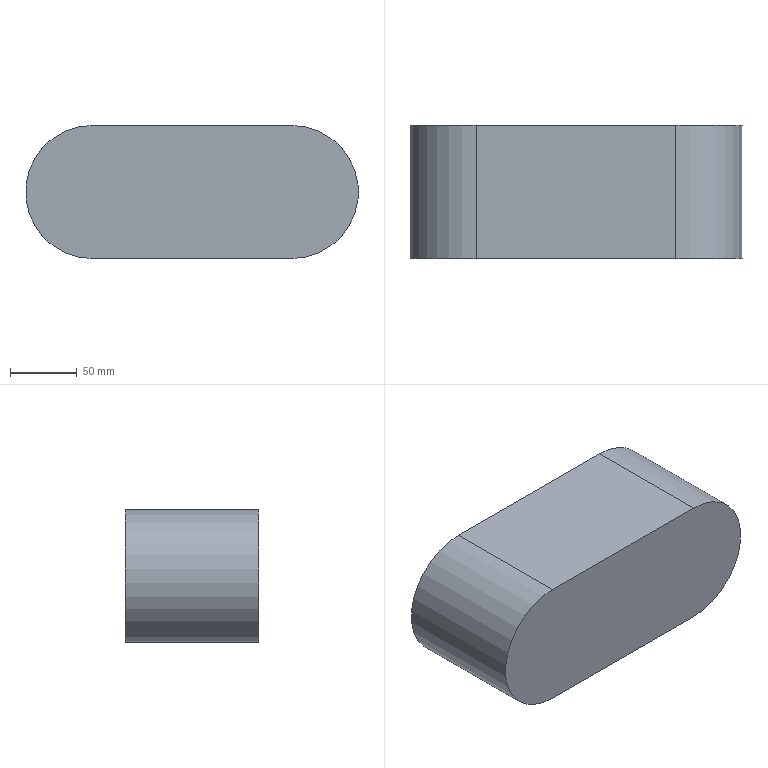Part | SolidWorks | features Extrusion 1 | 1 solid | 6 faces | box 250 x 100 x 100 mm | volume 2285398 mm3 | plane 4 | cylinder 2 | commonest cylinder face diameters 100 x2
STEP:
#1=CARTESIAN_POINT('',(-75.,0.,-50.));
#2=VERTEX_POINT('',#1);
#3=CARTESIAN_POINT('',(-75.,0.,50.));
#4=VERTEX_POINT('',#3);
#5=CARTESIAN_POINT('',(-75.,0.,0.));
#6=DIRECTION('',(0.,1.,0.));
#7=DIRECTION('',(0.,0.,1.));
#8=AXIS2_PLACEMENT_3D('',#5,#6,#7);
#9=CIRCLE('',#8,50.);
#10=EDGE_CURVE('',#2,#4,#9,.T.);
#11=ORIENTED_EDGE('',*,*,#10,.T.);
#12=CARTESIAN_POINT('',(-75.,100.,50.));
#13=VERTEX_POINT('',#12);
#14=CARTESIAN_POINT('',(-75.,100.,50.));
#15=DIRECTION('',(0.,-1.,0.));
#16=VECTOR('',#15,1000.);
#17=LINE('',#14,#16);
#18=EDGE_CURVE('',#13,#4,#17,.T.);
#19=ORIENTED_EDGE('',*,*,#18,.F.);
#20=CARTESIAN_POINT('',(-75.,100.,-50.));
#21=VERTEX_POINT('',#20);
#22=CARTESIAN_POINT('',(-75.,100.,0.));
#23=DIRECTION('',(0.,1.,0.));
#24=DIRECTION('',(0.,0.,1.));
#25=AXIS2_PLACEMENT_3D('',#22,#23,#24);
#26=CIRCLE('',#25,50.);
#27=EDGE_CURVE('',#21,#13,#26,.T.);
#28=ORIENTED_EDGE('',*,*,#27,.F.);
#29=CARTESIAN_POINT('',(-75.,100.,-50.));
#30=DIRECTION('',(0.,-1.,0.));
#31=VECTOR('',#30,1000.);
#32=LINE('',#29,#31);
#33=EDGE_CURVE('',#21,#2,#32,.T.);
#34=ORIENTED_EDGE('',*,*,#33,.T.);
#35=EDGE_LOOP('',(#11,#19,#28,#34));
#36=FACE_OUTER_BOUND('',#35,.T.);
#37=CARTESIAN_POINT('',(-75.,100.,0.));
#38=DIRECTION('',(0.,-1.,0.));
#39=DIRECTION('',(0.,0.,-1.));
#40=AXIS2_PLACEMENT_3D('',#37,#38,#39);
#41=CYLINDRICAL_SURFACE('',#40,50.);
#42=ADVANCED_FACE('',(#36),#41,.T.);
#43=CARTESIAN_POINT('',(75.,0.,50.));
#44=VERTEX_POINT('',#43);
#45=CARTESIAN_POINT('',(-75.,0.,50.));
#46=DIRECTION('',(1.,0.,0.));
#47=VECTOR('',#46,1000.);
#48=LINE('',#45,#47);
#49=EDGE_CURVE('',#4,#44,#48,.T.);
#50=ORIENTED_EDGE('',*,*,#49,.T.);
#51=CARTESIAN_POINT('',(75.,100.,50.));
#52=VERTEX_POINT('',#51);
#53=CARTESIAN_POINT('',(75.,100.,50.));
#54=DIRECTION('',(0.,-1.,0.));
#55=VECTOR('',#54,1000.);
#56=LINE('',#53,#55);
#57=EDGE_CURVE('',#52,#44,#56,.T.);
#58=ORIENTED_EDGE('',*,*,#57,.F.);
#59=CARTESIAN_POINT('',(-75.,100.,50.));
#60=DIRECTION('',(1.,0.,0.));
#61=VECTOR('',#60,1000.);
#62=LINE('',#59,#61);
#63=EDGE_CURVE('',#13,#52,#62,.T.);
#64=ORIENTED_EDGE('',*,*,#63,.F.);
#65=ORIENTED_EDGE('',*,*,#18,.T.);
#66=EDGE_LOOP('',(#50,#58,#64,#65));
#67=FACE_OUTER_BOUND('',#66,.T.);
#68=CARTESIAN_POINT('',(-75.,100.,50.));
#69=DIRECTION('',(0.,0.,-1.));
#70=DIRECTION('',(-1.,0.,0.));
#71=AXIS2_PLACEMENT_3D('',#68,#69,#70);
#72=PLANE('',#71);
#73=ADVANCED_FACE('',(#67),#72,.F.);
#74=CARTESIAN_POINT('',(75.,0.,-50.));
#75=VERTEX_POINT('',#74);
#76=CARTESIAN_POINT('',(75.,0.,0.));
#77=DIRECTION('',(0.,1.,0.));
#78=DIRECTION('',(0.,0.,1.));
#79=AXIS2_PLACEMENT_3D('',#76,#77,#78);
#80=CIRCLE('',#79,50.);
#81=EDGE_CURVE('',#44,#75,#80,.T.);
#82=ORIENTED_EDGE('',*,*,#81,.T.);
#83=CARTESIAN_POINT('',(75.,100.,-50.));
#84=VERTEX_POINT('',#83);
#85=CARTESIAN_POINT('',(75.,100.,-50.));
#86=DIRECTION('',(0.,-1.,0.));
#87=VECTOR('',#86,1000.);
#88=LINE('',#85,#87);
#89=EDGE_CURVE('',#84,#75,#88,.T.);
#90=ORIENTED_EDGE('',*,*,#89,.F.);
#91=CARTESIAN_POINT('',(75.,100.,0.));
#92=DIRECTION('',(0.,1.,0.));
#93=DIRECTION('',(0.,0.,1.));
#94=AXIS2_PLACEMENT_3D('',#91,#92,#93);
#95=CIRCLE('',#94,50.);
#96=EDGE_CURVE('',#52,#84,#95,.T.);
#97=ORIENTED_EDGE('',*,*,#96,.F.);
#98=ORIENTED_EDGE('',*,*,#57,.T.);
#99=EDGE_LOOP('',(#82,#90,#97,#98));
#100=FACE_OUTER_BOUND('',#99,.T.);
#101=CARTESIAN_POINT('',(75.,100.,0.));
#102=DIRECTION('',(0.,-1.,0.));
#103=DIRECTION('',(0.,0.,-1.));
#104=AXIS2_PLACEMENT_3D('',#101,#102,#103);
#105=CYLINDRICAL_SURFACE('',#104,50.);
#106=ADVANCED_FACE('',(#100),#105,.T.);
#107=CARTESIAN_POINT('',(-75.,0.,-50.));
#108=DIRECTION('',(-1.,0.,0.));
#109=VECTOR('',#108,1000.);
#110=LINE('',#107,#109);
#111=EDGE_CURVE('',#75,#2,#110,.T.);
#112=ORIENTED_EDGE('',*,*,#111,.T.);
#113=ORIENTED_EDGE('',*,*,#33,.F.);
#114=CARTESIAN_POINT('',(-75.,100.,-50.));
#115=DIRECTION('',(-1.,0.,0.));
#116=VECTOR('',#115,1000.);
#117=LINE('',#114,#116);
#118=EDGE_CURVE('',#84,#21,#117,.T.);
#119=ORIENTED_EDGE('',*,*,#118,.F.);
#120=ORIENTED_EDGE('',*,*,#89,.T.);
#121=EDGE_LOOP('',(#112,#113,#119,#120));
#122=FACE_OUTER_BOUND('',#121,.T.);
#123=CARTESIAN_POINT('',(-75.,100.,-50.));
#124=DIRECTION('',(0.,0.,1.));
#125=DIRECTION('',(1.,0.,0.));
#126=AXIS2_PLACEMENT_3D('',#123,#124,#125);
#127=PLANE('',#126);
#128=ADVANCED_FACE('',(#122),#127,.F.);
#129=ORIENTED_EDGE('',*,*,#27,.T.);
#130=ORIENTED_EDGE('',*,*,#63,.T.);
#131=ORIENTED_EDGE('',*,*,#96,.T.);
#132=ORIENTED_EDGE('',*,*,#118,.T.);
#133=EDGE_LOOP('',(#129,#130,#131,#132));
#134=FACE_OUTER_BOUND('',#133,.T.);
#135=CARTESIAN_POINT('',(-75.,100.,0.));
#136=DIRECTION('',(0.,1.,0.));
#137=DIRECTION('',(0.,0.,1.));
#138=AXIS2_PLACEMENT_3D('',#135,#136,#137);
#139=PLANE('',#138);
#140=ADVANCED_FACE('',(#134),#139,.T.);
#141=ORIENTED_EDGE('',*,*,#10,.F.);
#142=ORIENTED_EDGE('',*,*,#111,.F.);
#143=ORIENTED_EDGE('',*,*,#81,.F.);
#144=ORIENTED_EDGE('',*,*,#49,.F.);
#145=EDGE_LOOP('',(#141,#142,#143,#144));
#146=FACE_OUTER_BOUND('',#145,.T.);
#147=CARTESIAN_POINT('',(-75.,0.,0.));
#148=DIRECTION('',(0.,1.,0.));
#149=DIRECTION('',(0.,0.,1.));
#150=AXIS2_PLACEMENT_3D('',#147,#148,#149);
#151=PLANE('',#150);
#152=ADVANCED_FACE('',(#146),#151,.F.);
#153=CLOSED_SHELL('',(#42,#73,#106,#128,#140,#152));
#154=MANIFOLD_SOLID_BREP('',#153);
#155=CARTESIAN_POINT('',(0.,0.,0.));
#156=DIRECTION('',(0.,0.,1.));
#157=DIRECTION('',(1.,0.,0.));
#158=AXIS2_PLACEMENT_3D('',#155,#156,#157);
#159=(LENGTH_UNIT()NAMED_UNIT(*)SI_UNIT(.MILLI.,.METRE.));
#160=UNCERTAINTY_MEASURE_WITH_UNIT(LENGTH_MEASURE(0.00001),#159,'','');
#161=(NAMED_UNIT(*)PLANE_ANGLE_UNIT()SI_UNIT($,.RADIAN.));
#162=(NAMED_UNIT(*)SI_UNIT($,.STERADIAN.)SOLID_ANGLE_UNIT());
#163=(GEOMETRIC_REPRESENTATION_CONTEXT(3)GLOBAL_UNCERTAINTY_ASSIGNED_CONTEXT((#160))GLOBAL_UNIT_ASSIGNED_CONTEXT((#159,#161,#162))REPRESENTATION_CONTEXT('',''));
#164=ADVANCED_BREP_SHAPE_REPRESENTATION('',(#154,#158),#163);